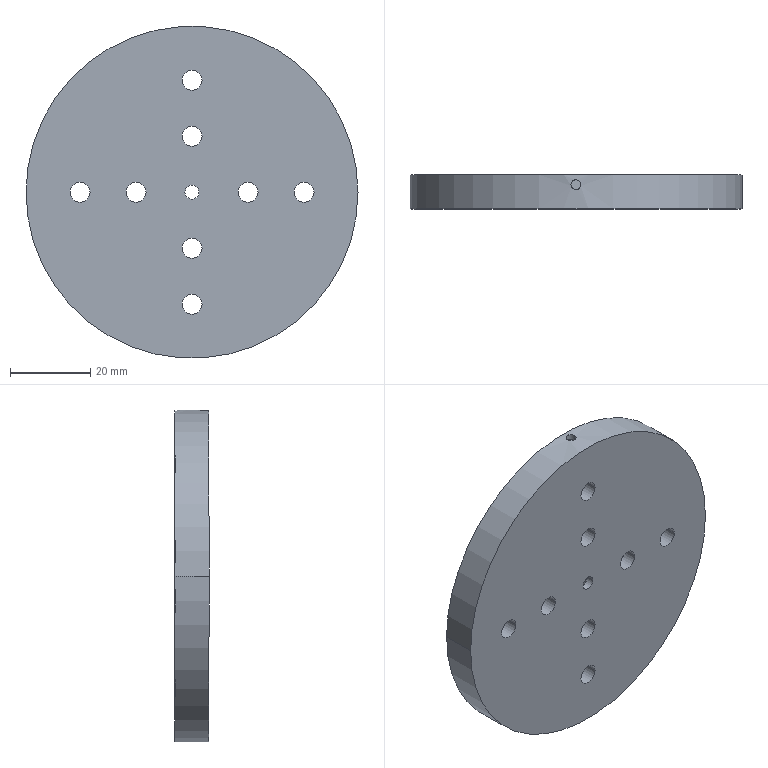Part | SolidWorks | features 3DProfileFeature 1, Chamfer 1, HoleWzd 1, ICE 1, Revolution 1 | 1 solid | 29 faces | box 83 x 8.5 x 83 mm | volume 20251 mm3 | cylinder 24 | plane 3 | cone 2 | commonest cylinder face diameters 5 x16 2.5 x2 3.5 x2 80 x2 83 x2
STEP:
#1=CARTESIAN_POINT('',(-1.25,6.,39.98));
#2=VERTEX_POINT('',#1);
#3=CARTESIAN_POINT('',(1.25,6.,39.98));
#4=VERTEX_POINT('',#3);
#5=CARTESIAN_POINT('',(-1.25,6.,39.98));
#6=CARTESIAN_POINT('',(-1.25,5.837,39.98));
#7=CARTESIAN_POINT('',(-1.217,5.672,39.982));
#8=CARTESIAN_POINT('',(-1.093,5.372,39.985));
#9=CARTESIAN_POINT('',(-0.9997,5.232,39.988));
#10=CARTESIAN_POINT('',(-0.7693,5.001,39.993));
#11=CARTESIAN_POINT('',(-0.6306,4.908,39.995));
#12=CARTESIAN_POINT('',(-0.3283,4.783,39.999));
#13=CARTESIAN_POINT('',(-0.1659,4.75,40.));
#14=CARTESIAN_POINT('',(0.1638,4.75,40.));
#15=CARTESIAN_POINT('',(0.3261,4.782,39.999));
#16=CARTESIAN_POINT('',(0.5535,4.876,39.996));
#17=CARTESIAN_POINT('',(0.6253,4.915,39.995));
#18=CARTESIAN_POINT('',(0.7611,5.005,39.993));
#19=CARTESIAN_POINT('',(0.8255,5.058,39.992));
#20=CARTESIAN_POINT('',(0.9987,5.231,39.988));
#21=CARTESIAN_POINT('',(1.092,5.37,39.985));
#22=CARTESIAN_POINT('',(1.217,5.671,39.982));
#23=CARTESIAN_POINT('',(1.25,5.835,39.98));
#24=CARTESIAN_POINT('',(1.25,6.,39.98));
#25=B_SPLINE_CURVE_WITH_KNOTS('',3,(#5,#6,#7,#8,#9,#10,#11,#12,#13,#14,#15,#16,#17,#18,#19,#20,#21,#22,#23,#24),.UNSPECIFIED.,.F.,.F.,(4,2,2,2,2,2,2,2,2,4),(0.003908,0.004397,0.004885,0.005374,0.005862,0.00635,0.006595,0.006839,0.007327,0.007816),.UNSPECIFIED.);
#26=EDGE_CURVE('',#2,#4,#25,.T.);
#27=ORIENTED_EDGE('',*,*,#26,.F.);
#28=CARTESIAN_POINT('',(-1.25,6.,41.481));
#29=VERTEX_POINT('',#28);
#30=CARTESIAN_POINT('',(-1.25,6.,41.5));
#31=DIRECTION('',(0.,0.,1.));
#32=VECTOR('',#31,1000.);
#33=LINE('',#30,#32);
#34=EDGE_CURVE('',#2,#29,#33,.T.);
#35=ORIENTED_EDGE('',*,*,#34,.T.);
#36=CARTESIAN_POINT('',(1.25,6.,41.481));
#37=VERTEX_POINT('',#36);
#38=CARTESIAN_POINT('',(1.25,6.,41.481));
#39=CARTESIAN_POINT('',(1.25,5.835,41.481));
#40=CARTESIAN_POINT('',(1.217,5.673,41.482));
#41=CARTESIAN_POINT('',(1.092,5.37,41.486));
#42=CARTESIAN_POINT('',(0.9991,5.231,41.488));
#43=CARTESIAN_POINT('',(0.7684,5.001,41.493));
#44=CARTESIAN_POINT('',(0.6289,4.908,41.496));
#45=CARTESIAN_POINT('',(0.328,4.783,41.499));
#46=CARTESIAN_POINT('',(0.1635,4.75,41.5));
#47=CARTESIAN_POINT('',(-0.1626,4.75,41.5));
#48=CARTESIAN_POINT('',(-0.3265,4.782,41.499));
#49=CARTESIAN_POINT('',(-0.6292,4.908,41.496));
#50=CARTESIAN_POINT('',(-0.767,4.999,41.493));
#51=CARTESIAN_POINT('',(-1.,5.233,41.488));
#52=CARTESIAN_POINT('',(-1.092,5.37,41.486));
#53=CARTESIAN_POINT('',(-1.186,5.597,41.483));
#54=CARTESIAN_POINT('',(-1.21,5.675,41.482));
#55=CARTESIAN_POINT('',(-1.242,5.836,41.481));
#56=CARTESIAN_POINT('',(-1.25,5.918,41.481));
#57=CARTESIAN_POINT('',(-1.25,6.,41.481));
#58=B_SPLINE_CURVE_WITH_KNOTS('',3,(#38,#39,#40,#41,#42,#43,#44,#45,#46,#47,#48,#49,#50,#51,#52,#53,#54,#55,#56,#57),.UNSPECIFIED.,.F.,.F.,(4,2,2,2,2,2,2,2,2,4),(0.,0.0004885,0.0009771,0.001466,0.001954,0.002443,0.002931,0.00342,0.003664,0.003908),.UNSPECIFIED.);
#59=EDGE_CURVE('',#37,#29,#58,.T.);
#60=ORIENTED_EDGE('',*,*,#59,.F.);
#61=CARTESIAN_POINT('',(1.25,6.,41.5));
#62=DIRECTION('',(0.,0.,1.));
#63=VECTOR('',#62,1000.);
#64=LINE('',#61,#63);
#65=EDGE_CURVE('',#4,#37,#64,.T.);
#66=ORIENTED_EDGE('',*,*,#65,.F.);
#67=EDGE_LOOP('',(#27,#35,#60,#66));
#68=FACE_OUTER_BOUND('',#67,.T.);
#69=CARTESIAN_POINT('',(0.,6.,41.5));
#70=DIRECTION('',(0.,0.,1.));
#71=DIRECTION('',(1.,0.,0.));
#72=AXIS2_PLACEMENT_3D('',#69,#70,#71);
#73=CYLINDRICAL_SURFACE('',#72,1.25);
#74=ADVANCED_FACE('',(#68),#73,.F.);
#75=CARTESIAN_POINT('',(-30.5,0.,0.));
#76=VERTEX_POINT('',#75);
#77=CARTESIAN_POINT('',(-25.5,0.,0.));
#78=VERTEX_POINT('',#77);
#79=CARTESIAN_POINT('',(-28.,0.,0.));
#80=DIRECTION('',(0.,-1.,0.));
#81=DIRECTION('',(-1.,0.,0.));
#82=AXIS2_PLACEMENT_3D('',#79,#80,#81);
#83=CIRCLE('',#82,2.5);
#84=EDGE_CURVE('',#76,#78,#83,.T.);
#85=ORIENTED_EDGE('',*,*,#84,.T.);
#86=CARTESIAN_POINT('',(-25.5,3.5,0.));
#87=VERTEX_POINT('',#86);
#88=CARTESIAN_POINT('',(-25.5,-0.001,0.));
#89=DIRECTION('',(0.,1.,0.));
#90=VECTOR('',#89,1000.);
#91=LINE('',#88,#90);
#92=EDGE_CURVE('',#78,#87,#91,.T.);
#93=ORIENTED_EDGE('',*,*,#92,.T.);
#94=CARTESIAN_POINT('',(-30.5,3.5,0.));
#95=VERTEX_POINT('',#94);
#96=CARTESIAN_POINT('',(-28.,3.5,0.));
#97=DIRECTION('',(0.,1.,0.));
#98=DIRECTION('',(-1.,0.,0.));
#99=AXIS2_PLACEMENT_3D('',#96,#97,#98);
#100=CIRCLE('',#99,2.5);
#101=EDGE_CURVE('',#87,#95,#100,.T.);
#102=ORIENTED_EDGE('',*,*,#101,.T.);
#103=CARTESIAN_POINT('',(-30.5,-0.001,0.));
#104=DIRECTION('',(0.,1.,0.));
#105=VECTOR('',#104,1000.);
#106=LINE('',#103,#105);
#107=EDGE_CURVE('',#76,#95,#106,.T.);
#108=ORIENTED_EDGE('',*,*,#107,.F.);
#109=EDGE_LOOP('',(#85,#93,#102,#108));
#110=FACE_OUTER_BOUND('',#109,.T.);
#111=CARTESIAN_POINT('',(-28.,-0.001,0.));
#112=DIRECTION('',(0.,1.,0.));
#113=DIRECTION('',(-1.,0.,0.));
#114=AXIS2_PLACEMENT_3D('',#111,#112,#113);
#115=CYLINDRICAL_SURFACE('',#114,2.5);
#116=ADVANCED_FACE('',(#110),#115,.F.);
#117=CARTESIAN_POINT('',(-16.5,0.,0.));
#118=VERTEX_POINT('',#117);
#119=CARTESIAN_POINT('',(-11.5,0.,0.));
#120=VERTEX_POINT('',#119);
#121=CARTESIAN_POINT('',(-14.,0.,0.));
#122=DIRECTION('',(0.,-1.,0.));
#123=DIRECTION('',(-1.,0.,0.));
#124=AXIS2_PLACEMENT_3D('',#121,#122,#123);
#125=CIRCLE('',#124,2.5);
#126=EDGE_CURVE('',#118,#120,#125,.T.);
#127=ORIENTED_EDGE('',*,*,#126,.T.);
#128=CARTESIAN_POINT('',(-11.5,3.5,0.));
#129=VERTEX_POINT('',#128);
#130=CARTESIAN_POINT('',(-11.5,-0.001,0.));
#131=DIRECTION('',(0.,1.,0.));
#132=VECTOR('',#131,1000.);
#133=LINE('',#130,#132);
#134=EDGE_CURVE('',#120,#129,#133,.T.);
#135=ORIENTED_EDGE('',*,*,#134,.T.);
#136=CARTESIAN_POINT('',(-16.5,3.5,0.));
#137=VERTEX_POINT('',#136);
#138=CARTESIAN_POINT('',(-14.,3.5,0.));
#139=DIRECTION('',(0.,1.,0.));
#140=DIRECTION('',(-1.,0.,0.));
#141=AXIS2_PLACEMENT_3D('',#138,#139,#140);
#142=CIRCLE('',#141,2.5);
#143=EDGE_CURVE('',#129,#137,#142,.T.);
#144=ORIENTED_EDGE('',*,*,#143,.T.);
#145=CARTESIAN_POINT('',(-16.5,-0.001,0.));
#146=DIRECTION('',(0.,1.,0.));
#147=VECTOR('',#146,1000.);
#148=LINE('',#145,#147);
#149=EDGE_CURVE('',#118,#137,#148,.T.);
#150=ORIENTED_EDGE('',*,*,#149,.F.);
#151=EDGE_LOOP('',(#127,#135,#144,#150));
#152=FACE_OUTER_BOUND('',#151,.T.);
#153=CARTESIAN_POINT('',(-14.,-0.001,0.));
#154=DIRECTION('',(0.,1.,0.));
#155=DIRECTION('',(-1.,0.,0.));
#156=AXIS2_PLACEMENT_3D('',#153,#154,#155);
#157=CYLINDRICAL_SURFACE('',#156,2.5);
#158=ADVANCED_FACE('',(#152),#157,.F.);
#159=CARTESIAN_POINT('',(-2.5,0.,28.));
#160=VERTEX_POINT('',#159);
#161=CARTESIAN_POINT('',(2.5,0.,28.));
#162=VERTEX_POINT('',#161);
#163=CARTESIAN_POINT('',(0.,0.,28.));
#164=DIRECTION('',(0.,-1.,0.));
#165=DIRECTION('',(-1.,0.,0.));
#166=AXIS2_PLACEMENT_3D('',#163,#164,#165);
#167=CIRCLE('',#166,2.5);
#168=EDGE_CURVE('',#160,#162,#167,.T.);
#169=ORIENTED_EDGE('',*,*,#168,.T.);
#170=CARTESIAN_POINT('',(2.5,3.5,28.));
#171=VERTEX_POINT('',#170);
#172=CARTESIAN_POINT('',(2.5,-0.001,28.));
#173=DIRECTION('',(0.,1.,0.));
#174=VECTOR('',#173,1000.);
#175=LINE('',#172,#174);
#176=EDGE_CURVE('',#162,#171,#175,.T.);
#177=ORIENTED_EDGE('',*,*,#176,.T.);
#178=CARTESIAN_POINT('',(-2.5,3.5,28.));
#179=VERTEX_POINT('',#178);
#180=CARTESIAN_POINT('',(0.,3.5,28.));
#181=DIRECTION('',(0.,1.,0.));
#182=DIRECTION('',(-1.,0.,0.));
#183=AXIS2_PLACEMENT_3D('',#180,#181,#182);
#184=CIRCLE('',#183,2.5);
#185=EDGE_CURVE('',#171,#179,#184,.T.);
#186=ORIENTED_EDGE('',*,*,#185,.T.);
#187=CARTESIAN_POINT('',(-2.5,-0.001,28.));
#188=DIRECTION('',(0.,1.,0.));
#189=VECTOR('',#188,1000.);
#190=LINE('',#187,#189);
#191=EDGE_CURVE('',#160,#179,#190,.T.);
#192=ORIENTED_EDGE('',*,*,#191,.F.);
#193=EDGE_LOOP('',(#169,#177,#186,#192));
#194=FACE_OUTER_BOUND('',#193,.T.);
#195=CARTESIAN_POINT('',(0.,-0.001,28.));
#196=DIRECTION('',(0.,1.,0.));
#197=DIRECTION('',(-1.,0.,0.));
#198=AXIS2_PLACEMENT_3D('',#195,#196,#197);
#199=CYLINDRICAL_SURFACE('',#198,2.5);
#200=ADVANCED_FACE('',(#194),#199,.F.);
#201=CARTESIAN_POINT('',(-2.5,0.,14.));
#202=VERTEX_POINT('',#201);
#203=CARTESIAN_POINT('',(2.5,0.,14.));
#204=VERTEX_POINT('',#203);
#205=CARTESIAN_POINT('',(0.,0.,14.));
#206=DIRECTION('',(0.,-1.,0.));
#207=DIRECTION('',(-1.,0.,0.));
#208=AXIS2_PLACEMENT_3D('',#205,#206,#207);
#209=CIRCLE('',#208,2.5);
#210=EDGE_CURVE('',#202,#204,#209,.T.);
#211=ORIENTED_EDGE('',*,*,#210,.T.);
#212=CARTESIAN_POINT('',(2.5,3.5,14.));
#213=VERTEX_POINT('',#212);
#214=CARTESIAN_POINT('',(2.5,-0.001,14.));
#215=DIRECTION('',(0.,1.,0.));
#216=VECTOR('',#215,1000.);
#217=LINE('',#214,#216);
#218=EDGE_CURVE('',#204,#213,#217,.T.);
#219=ORIENTED_EDGE('',*,*,#218,.T.);
#220=CARTESIAN_POINT('',(-2.5,3.5,14.));
#221=VERTEX_POINT('',#220);
#222=CARTESIAN_POINT('',(0.,3.5,14.));
#223=DIRECTION('',(0.,1.,0.));
#224=DIRECTION('',(-1.,0.,0.));
#225=AXIS2_PLACEMENT_3D('',#222,#223,#224);
#226=CIRCLE('',#225,2.5);
#227=EDGE_CURVE('',#213,#221,#226,.T.);
#228=ORIENTED_EDGE('',*,*,#227,.T.);
#229=CARTESIAN_POINT('',(-2.5,-0.001,14.));
#230=DIRECTION('',(0.,1.,0.));
#231=VECTOR('',#230,1000.);
#232=LINE('',#229,#231);
#233=EDGE_CURVE('',#202,#221,#232,.T.);
#234=ORIENTED_EDGE('',*,*,#233,.F.);
#235=EDGE_LOOP('',(#211,#219,#228,#234));
#236=FACE_OUTER_BOUND('',#235,.T.);
#237=CARTESIAN_POINT('',(0.,-0.001,14.));
#238=DIRECTION('',(0.,1.,0.));
#239=DIRECTION('',(-1.,0.,0.));
#240=AXIS2_PLACEMENT_3D('',#237,#238,#239);
#241=CYLINDRICAL_SURFACE('',#240,2.5);
#242=ADVANCED_FACE('',(#236),#241,.F.);
#243=CARTESIAN_POINT('',(25.5,0.,0.));
#244=VERTEX_POINT('',#243);
#245=CARTESIAN_POINT('',(30.5,0.,0.));
#246=VERTEX_POINT('',#245);
#247=CARTESIAN_POINT('',(28.,0.,0.));
#248=DIRECTION('',(0.,-1.,0.));
#249=DIRECTION('',(-1.,0.,0.));
#250=AXIS2_PLACEMENT_3D('',#247,#248,#249);
#251=CIRCLE('',#250,2.5);
#252=EDGE_CURVE('',#244,#246,#251,.T.);
#253=ORIENTED_EDGE('',*,*,#252,.T.);
#254=CARTESIAN_POINT('',(30.5,3.5,0.));
#255=VERTEX_POINT('',#254);
#256=CARTESIAN_POINT('',(30.5,-0.001,0.));
#257=DIRECTION('',(0.,1.,0.));
#258=VECTOR('',#257,1000.);
#259=LINE('',#256,#258);
#260=EDGE_CURVE('',#246,#255,#259,.T.);
#261=ORIENTED_EDGE('',*,*,#260,.T.);
#262=CARTESIAN_POINT('',(25.5,3.5,0.));
#263=VERTEX_POINT('',#262);
#264=CARTESIAN_POINT('',(28.,3.5,0.));
#265=DIRECTION('',(0.,1.,0.));
#266=DIRECTION('',(-1.,0.,0.));
#267=AXIS2_PLACEMENT_3D('',#264,#265,#266);
#268=CIRCLE('',#267,2.5);
#269=EDGE_CURVE('',#255,#263,#268,.T.);
#270=ORIENTED_EDGE('',*,*,#269,.T.);
#271=CARTESIAN_POINT('',(25.5,-0.001,0.));
#272=DIRECTION('',(0.,1.,0.));
#273=VECTOR('',#272,1000.);
#274=LINE('',#271,#273);
#275=EDGE_CURVE('',#244,#263,#274,.T.);
#276=ORIENTED_EDGE('',*,*,#275,.F.);
#277=EDGE_LOOP('',(#253,#261,#270,#276));
#278=FACE_OUTER_BOUND('',#277,.T.);
#279=CARTESIAN_POINT('',(28.,-0.001,0.));
#280=DIRECTION('',(0.,1.,0.));
#281=DIRECTION('',(-1.,0.,0.));
#282=AXIS2_PLACEMENT_3D('',#279,#280,#281);
#283=CYLINDRICAL_SURFACE('',#282,2.5);
#284=ADVANCED_FACE('',(#278),#283,.F.);
#285=CARTESIAN_POINT('',(11.5,0.,0.));
#286=VERTEX_POINT('',#285);
#287=CARTESIAN_POINT('',(16.5,0.,0.));
#288=VERTEX_POINT('',#287);
#289=CARTESIAN_POINT('',(14.,0.,0.));
#290=DIRECTION('',(0.,-1.,0.));
#291=DIRECTION('',(-1.,0.,0.));
#292=AXIS2_PLACEMENT_3D('',#289,#290,#291);
#293=CIRCLE('',#292,2.5);
#294=EDGE_CURVE('',#286,#288,#293,.T.);
#295=ORIENTED_EDGE('',*,*,#294,.T.);
#296=CARTESIAN_POINT('',(16.5,3.5,0.));
#297=VERTEX_POINT('',#296);
#298=CARTESIAN_POINT('',(16.5,-0.001,0.));
#299=DIRECTION('',(0.,1.,0.));
#300=VECTOR('',#299,1000.);
#301=LINE('',#298,#300);
#302=EDGE_CURVE('',#288,#297,#301,.T.);
#303=ORIENTED_EDGE('',*,*,#302,.T.);
#304=CARTESIAN_POINT('',(11.5,3.5,0.));
#305=VERTEX_POINT('',#304);
#306=CARTESIAN_POINT('',(14.,3.5,0.));
#307=DIRECTION('',(0.,1.,0.));
#308=DIRECTION('',(-1.,0.,0.));
#309=AXIS2_PLACEMENT_3D('',#306,#307,#308);
#310=CIRCLE('',#309,2.5);
#311=EDGE_CURVE('',#297,#305,#310,.T.);
#312=ORIENTED_EDGE('',*,*,#311,.T.);
#313=CARTESIAN_POINT('',(11.5,-0.001,0.));
#314=DIRECTION('',(0.,1.,0.));
#315=VECTOR('',#314,1000.);
#316=LINE('',#313,#315);
#317=EDGE_CURVE('',#286,#305,#316,.T.);
#318=ORIENTED_EDGE('',*,*,#317,.F.);
#319=EDGE_LOOP('',(#295,#303,#312,#318));
#320=FACE_OUTER_BOUND('',#319,.T.);
#321=CARTESIAN_POINT('',(14.,-0.001,0.));
#322=DIRECTION('',(0.,1.,0.));
#323=DIRECTION('',(-1.,0.,0.));
#324=AXIS2_PLACEMENT_3D('',#321,#322,#323);
#325=CYLINDRICAL_SURFACE('',#324,2.5);
#326=ADVANCED_FACE('',(#320),#325,.F.);
#327=CARTESIAN_POINT('',(-2.5,0.,-28.));
#328=VERTEX_POINT('',#327);
#329=CARTESIAN_POINT('',(2.5,0.,-28.));
#330=VERTEX_POINT('',#329);
#331=CARTESIAN_POINT('',(0.,0.,-28.));
#332=DIRECTION('',(0.,-1.,0.));
#333=DIRECTION('',(-1.,0.,0.));
#334=AXIS2_PLACEMENT_3D('',#331,#332,#333);
#335=CIRCLE('',#334,2.5);
#336=EDGE_CURVE('',#328,#330,#335,.T.);
#337=ORIENTED_EDGE('',*,*,#336,.T.);
#338=CARTESIAN_POINT('',(2.5,3.5,-28.));
#339=VERTEX_POINT('',#338);
#340=CARTESIAN_POINT('',(2.5,-0.001,-28.));
#341=DIRECTION('',(0.,1.,0.));
#342=VECTOR('',#341,1000.);
#343=LINE('',#340,#342);
#344=EDGE_CURVE('',#330,#339,#343,.T.);
#345=ORIENTED_EDGE('',*,*,#344,.T.);
#346=CARTESIAN_POINT('',(-2.5,3.5,-28.));
#347=VERTEX_POINT('',#346);
#348=CARTESIAN_POINT('',(0.,3.5,-28.));
#349=DIRECTION('',(0.,1.,0.));
#350=DIRECTION('',(-1.,0.,0.));
#351=AXIS2_PLACEMENT_3D('',#348,#349,#350);
#352=CIRCLE('',#351,2.5);
#353=EDGE_CURVE('',#339,#347,#352,.T.);
#354=ORIENTED_EDGE('',*,*,#353,.T.);
#355=CARTESIAN_POINT('',(-2.5,-0.001,-28.));
#356=DIRECTION('',(0.,1.,0.));
#357=VECTOR('',#356,1000.);
#358=LINE('',#355,#357);
#359=EDGE_CURVE('',#328,#347,#358,.T.);
#360=ORIENTED_EDGE('',*,*,#359,.F.);
#361=EDGE_LOOP('',(#337,#345,#354,#360));
#362=FACE_OUTER_BOUND('',#361,.T.);
#363=CARTESIAN_POINT('',(0.,-0.001,-28.));
#364=DIRECTION('',(0.,1.,0.));
#365=DIRECTION('',(-1.,0.,0.));
#366=AXIS2_PLACEMENT_3D('',#363,#364,#365);
#367=CYLINDRICAL_SURFACE('',#366,2.5);
#368=ADVANCED_FACE('',(#362),#367,.F.);
#369=CARTESIAN_POINT('',(-2.5,0.,-14.));
#370=VERTEX_POINT('',#369);
#371=CARTESIAN_POINT('',(2.5,0.,-14.));
#372=VERTEX_POINT('',#371);
#373=CARTESIAN_POINT('',(0.,0.,-14.));
#374=DIRECTION('',(0.,-1.,0.));
#375=DIRECTION('',(-1.,0.,0.));
#376=AXIS2_PLACEMENT_3D('',#373,#374,#375);
#377=CIRCLE('',#376,2.5);
#378=EDGE_CURVE('',#370,#372,#377,.T.);
#379=ORIENTED_EDGE('',*,*,#378,.T.);
#380=CARTESIAN_POINT('',(2.5,3.5,-14.));
#381=VERTEX_POINT('',#380);
#382=CARTESIAN_POINT('',(2.5,-0.001,-14.));
#383=DIRECTION('',(0.,1.,0.));
#384=VECTOR('',#383,1000.);
#385=LINE('',#382,#384);
#386=EDGE_CURVE('',#372,#381,#385,.T.);
#387=ORIENTED_EDGE('',*,*,#386,.T.);
#388=CARTESIAN_POINT('',(-2.5,3.5,-14.));
#389=VERTEX_POINT('',#388);
#390=CARTESIAN_POINT('',(0.,3.5,-14.));
#391=DIRECTION('',(0.,1.,0.));
#392=DIRECTION('',(-1.,0.,0.));
#393=AXIS2_PLACEMENT_3D('',#390,#391,#392);
#394=CIRCLE('',#393,2.5);
#395=EDGE_CURVE('',#381,#389,#394,.T.);
#396=ORIENTED_EDGE('',*,*,#395,.T.);
#397=CARTESIAN_POINT('',(-2.5,-0.001,-14.));
#398=DIRECTION('',(0.,1.,0.));
#399=VECTOR('',#398,1000.);
#400=LINE('',#397,#399);
#401=EDGE_CURVE('',#370,#389,#400,.T.);
#402=ORIENTED_EDGE('',*,*,#401,.F.);
#403=EDGE_LOOP('',(#379,#387,#396,#402));
#404=FACE_OUTER_BOUND('',#403,.T.);
#405=CARTESIAN_POINT('',(0.,-0.001,-14.));
#406=DIRECTION('',(0.,1.,0.));
#407=DIRECTION('',(-1.,0.,0.));
#408=AXIS2_PLACEMENT_3D('',#405,#406,#407);
#409=CYLINDRICAL_SURFACE('',#408,2.5);
#410=ADVANCED_FACE('',(#404),#409,.F.);
#411=ORIENTED_EDGE('',*,*,#59,.T.);
#412=CARTESIAN_POINT('',(-1.25,6.,41.481));
#413=CARTESIAN_POINT('',(-1.25,6.163,41.481));
#414=CARTESIAN_POINT('',(-1.217,6.328,41.482));
#415=CARTESIAN_POINT('',(-1.093,6.628,41.486));
#416=CARTESIAN_POINT('',(-0.9997,6.768,41.488));
#417=CARTESIAN_POINT('',(-0.7693,6.999,41.493));
#418=CARTESIAN_POINT('',(-0.6306,7.092,41.495));
#419=CARTESIAN_POINT('',(-0.3283,7.217,41.499));
#420=CARTESIAN_POINT('',(-0.1659,7.25,41.5));
#421=CARTESIAN_POINT('',(0.1638,7.25,41.5));
#422=CARTESIAN_POINT('',(0.3261,7.218,41.499));
#423=CARTESIAN_POINT('',(0.5535,7.124,41.496));
#424=CARTESIAN_POINT('',(0.6253,7.085,41.495));
#425=CARTESIAN_POINT('',(0.7611,6.995,41.493));
#426=CARTESIAN_POINT('',(0.8255,6.942,41.492));
#427=CARTESIAN_POINT('',(0.9987,6.769,41.488));
#428=CARTESIAN_POINT('',(1.092,6.63,41.486));
#429=CARTESIAN_POINT('',(1.217,6.329,41.482));
#430=CARTESIAN_POINT('',(1.25,6.165,41.481));
#431=CARTESIAN_POINT('',(1.25,6.,41.481));
#432=B_SPLINE_CURVE_WITH_KNOTS('',3,(#412,#413,#414,#415,#416,#417,#418,#419,#420,#421,#422,#423,#424,#425,#426,#427,#428,#429,#430,#431),.UNSPECIFIED.,.F.,.F.,(4,2,2,2,2,2,2,2,2,4),(0.003908,0.004397,0.004885,0.005374,0.005862,0.00635,0.006595,0.006839,0.007327,0.007816),.UNSPECIFIED.);
#433=EDGE_CURVE('',#29,#37,#432,.T.);
#434=ORIENTED_EDGE('',*,*,#433,.T.);
#435=EDGE_LOOP('',(#411,#434));
#436=FACE_BOUND('',#435,.T.);
#437=CARTESIAN_POINT('',(-41.5,0.,0.));
#438=VERTEX_POINT('',#437);
#439=CARTESIAN_POINT('',(41.5,0.,0.));
#440=VERTEX_POINT('',#439);
#441=CARTESIAN_POINT('',(0.,0.,0.));
#442=DIRECTION('',(0.,1.,0.));
#443=DIRECTION('',(-1.,0.,0.));
#444=AXIS2_PLACEMENT_3D('',#441,#442,#443);
#445=CIRCLE('',#444,41.5);
#446=EDGE_CURVE('',#438,#440,#445,.T.);
#447=ORIENTED_EDGE('',*,*,#446,.T.);
#448=CARTESIAN_POINT('',(41.5,8.5,0.));
#449=VERTEX_POINT('',#448);
#450=CARTESIAN_POINT('',(41.5,9.31,0.));
#451=DIRECTION('',(0.,1.,0.));
#452=VECTOR('',#451,1000.);
#453=LINE('',#450,#452);
#454=EDGE_CURVE('',#440,#449,#453,.T.);
#455=ORIENTED_EDGE('',*,*,#454,.T.);
#456=CARTESIAN_POINT('',(-41.5,8.5,0.));
#457=VERTEX_POINT('',#456);
#458=CARTESIAN_POINT('',(0.,8.5,0.));
#459=DIRECTION('',(0.,1.,0.));
#460=DIRECTION('',(-1.,0.,0.));
#461=AXIS2_PLACEMENT_3D('',#458,#459,#460);
#462=CIRCLE('',#461,41.5);
#463=EDGE_CURVE('',#457,#449,#462,.T.);
#464=ORIENTED_EDGE('',*,*,#463,.F.);
#465=CARTESIAN_POINT('',(-41.5,9.31,0.));
#466=DIRECTION('',(0.,1.,0.));
#467=VECTOR('',#466,1000.);
#468=LINE('',#465,#467);
#469=EDGE_CURVE('',#438,#457,#468,.T.);
#470=ORIENTED_EDGE('',*,*,#469,.F.);
#471=EDGE_LOOP('',(#447,#455,#464,#470));
#472=FACE_OUTER_BOUND('',#471,.T.);
#473=CARTESIAN_POINT('',(0.,9.31,0.));
#474=DIRECTION('',(0.,1.,0.));
#475=DIRECTION('',(-1.,0.,0.));
#476=AXIS2_PLACEMENT_3D('',#473,#474,#475);
#477=CYLINDRICAL_SURFACE('',#476,41.5);
#478=ADVANCED_FACE('',(#436,#472),#477,.T.);
#479=CARTESIAN_POINT('',(40.,3.5,0.));
#480=VERTEX_POINT('',#479);
#481=CARTESIAN_POINT('',(-40.,3.5,0.));
#482=VERTEX_POINT('',#481);
#483=CARTESIAN_POINT('',(0.,3.5,0.));
#484=DIRECTION('',(0.,1.,0.));
#485=DIRECTION('',(-1.,0.,0.));
#486=AXIS2_PLACEMENT_3D('',#483,#484,#485);
#487=CIRCLE('',#486,40.);
#488=EDGE_CURVE('',#480,#482,#487,.T.);
#489=ORIENTED_EDGE('',*,*,#488,.F.);
#490=CARTESIAN_POINT('',(40.,8.5,0.));
#491=VERTEX_POINT('',#490);
#492=CARTESIAN_POINT('',(40.,9.31,0.));
#493=DIRECTION('',(0.,1.,0.));
#494=VECTOR('',#493,1000.);
#495=LINE('',#492,#494);
#496=EDGE_CURVE('',#480,#491,#495,.T.);
#497=ORIENTED_EDGE('',*,*,#496,.T.);
#498=CARTESIAN_POINT('',(-40.,8.5,0.));
#499=VERTEX_POINT('',#498);
#500=CARTESIAN_POINT('',(0.,8.5,0.));
#501=DIRECTION('',(0.,1.,0.));
#502=DIRECTION('',(-1.,0.,0.));
#503=AXIS2_PLACEMENT_3D('',#500,#501,#502);
#504=CIRCLE('',#503,40.);
#505=EDGE_CURVE('',#491,#499,#504,.T.);
#506=ORIENTED_EDGE('',*,*,#505,.T.);
#507=CARTESIAN_POINT('',(-40.,9.31,0.));
#508=DIRECTION('',(0.,1.,0.));
#509=VECTOR('',#508,1000.);
#510=LINE('',#507,#509);
#511=EDGE_CURVE('',#482,#499,#510,.T.);
#512=ORIENTED_EDGE('',*,*,#511,.F.);
#513=EDGE_LOOP('',(#489,#497,#506,#512));
#514=FACE_OUTER_BOUND('',#513,.T.);
#515=CARTESIAN_POINT('',(0.,9.31,0.));
#516=DIRECTION('',(0.,1.,0.));
#517=DIRECTION('',(-1.,0.,0.));
#518=AXIS2_PLACEMENT_3D('',#515,#516,#517);
#519=CYLINDRICAL_SURFACE('',#518,40.);
#520=ADVANCED_FACE('',(#514),#519,.F.);
#521=CARTESIAN_POINT('',(1.75,2.,0.));
#522=VERTEX_POINT('',#521);
#523=CARTESIAN_POINT('',(-1.75,2.,0.));
#524=VERTEX_POINT('',#523);
#525=CARTESIAN_POINT('',(0.,2.,0.));
#526=DIRECTION('',(0.,1.,0.));
#527=DIRECTION('',(-1.,0.,0.));
#528=AXIS2_PLACEMENT_3D('',#525,#526,#527);
#529=CIRCLE('',#528,1.75);
#530=EDGE_CURVE('',#522,#524,#529,.T.);
#531=ORIENTED_EDGE('',*,*,#530,.F.);
#532=CARTESIAN_POINT('',(3.25,3.5,0.));
#533=VERTEX_POINT('',#532);
#534=CARTESIAN_POINT('',(3.25,3.5,0.));
#535=DIRECTION('',(0.7071,0.7071,0.));
#536=VECTOR('',#535,1000.);
#537=LINE('',#534,#536);
#538=EDGE_CURVE('',#522,#533,#537,.T.);
#539=ORIENTED_EDGE('',*,*,#538,.T.);
#540=CARTESIAN_POINT('',(-3.25,3.5,0.));
#541=VERTEX_POINT('',#540);
#542=CARTESIAN_POINT('',(0.,3.5,0.));
#543=DIRECTION('',(0.,1.,0.));
#544=DIRECTION('',(-1.,0.,0.));
#545=AXIS2_PLACEMENT_3D('',#542,#543,#544);
#546=CIRCLE('',#545,3.25);
#547=EDGE_CURVE('',#533,#541,#546,.T.);
#548=ORIENTED_EDGE('',*,*,#547,.T.);
#549=CARTESIAN_POINT('',(-3.25,3.5,0.));
#550=DIRECTION('',(-0.7071,0.7071,0.));
#551=VECTOR('',#550,1000.);
#552=LINE('',#549,#551);
#553=EDGE_CURVE('',#524,#541,#552,.T.);
#554=ORIENTED_EDGE('',*,*,#553,.F.);
#555=EDGE_LOOP('',(#531,#539,#548,#554));
#556=FACE_OUTER_BOUND('',#555,.T.);
#557=CARTESIAN_POINT('',(0.,3.5,0.));
#558=DIRECTION('',(0.,1.,0.));
#559=DIRECTION('',(-1.,0.,0.));
#560=AXIS2_PLACEMENT_3D('',#557,#558,#559);
#561=CONICAL_SURFACE('',#560,3.25,0.7854);
#562=ADVANCED_FACE('',(#556),#561,.F.);
#563=CARTESIAN_POINT('',(1.75,0.,0.));
#564=VERTEX_POINT('',#563);
#565=CARTESIAN_POINT('',(-1.75,0.,0.));
#566=VERTEX_POINT('',#565);
#567=CARTESIAN_POINT('',(0.,0.,0.));
#568=DIRECTION('',(0.,1.,0.));
#569=DIRECTION('',(-1.,0.,0.));
#570=AXIS2_PLACEMENT_3D('',#567,#568,#569);
#571=CIRCLE('',#570,1.75);
#572=EDGE_CURVE('',#564,#566,#571,.T.);
#573=ORIENTED_EDGE('',*,*,#572,.F.);
#574=CARTESIAN_POINT('',(1.75,9.31,0.));
#575=DIRECTION('',(0.,1.,0.));
#576=VECTOR('',#575,1000.);
#577=LINE('',#574,#576);
#578=EDGE_CURVE('',#564,#522,#577,.T.);
#579=ORIENTED_EDGE('',*,*,#578,.T.);
#580=ORIENTED_EDGE('',*,*,#530,.T.);
#581=CARTESIAN_POINT('',(-1.75,9.31,0.));
#582=DIRECTION('',(0.,1.,0.));
#583=VECTOR('',#582,1000.);
#584=LINE('',#581,#583);
#585=EDGE_CURVE('',#566,#524,#584,.T.);
#586=ORIENTED_EDGE('',*,*,#585,.F.);
#587=EDGE_LOOP('',(#573,#579,#580,#586));
#588=FACE_OUTER_BOUND('',#587,.T.);
#589=CARTESIAN_POINT('',(0.,9.31,0.));
#590=DIRECTION('',(0.,1.,0.));
#591=DIRECTION('',(-1.,0.,0.));
#592=AXIS2_PLACEMENT_3D('',#589,#590,#591);
#593=CYLINDRICAL_SURFACE('',#592,1.75);
#594=ADVANCED_FACE('',(#588),#593,.F.);
#595=ORIENTED_EDGE('',*,*,#84,.F.);
#596=CARTESIAN_POINT('',(-28.,0.,0.));
#597=DIRECTION('',(0.,-1.,0.));
#598=DIRECTION('',(-1.,0.,0.));
#599=AXIS2_PLACEMENT_3D('',#596,#597,#598);
#600=CIRCLE('',#599,2.5);
#601=EDGE_CURVE('',#78,#76,#600,.T.);
#602=ORIENTED_EDGE('',*,*,#601,.F.);
#603=EDGE_LOOP('',(#595,#602));
#604=FACE_BOUND('',#603,.T.);
#605=ORIENTED_EDGE('',*,*,#126,.F.);
#606=CARTESIAN_POINT('',(-14.,0.,0.));
#607=DIRECTION('',(0.,-1.,0.));
#608=DIRECTION('',(-1.,0.,0.));
#609=AXIS2_PLACEMENT_3D('',#606,#607,#608);
#610=CIRCLE('',#609,2.5);
#611=EDGE_CURVE('',#120,#118,#610,.T.);
#612=ORIENTED_EDGE('',*,*,#611,.F.);
#613=EDGE_LOOP('',(#605,#612));
#614=FACE_BOUND('',#613,.T.);
#615=ORIENTED_EDGE('',*,*,#168,.F.);
#616=CARTESIAN_POINT('',(0.,0.,28.));
#617=DIRECTION('',(0.,-1.,0.));
#618=DIRECTION('',(-1.,0.,0.));
#619=AXIS2_PLACEMENT_3D('',#616,#617,#618);
#620=CIRCLE('',#619,2.5);
#621=EDGE_CURVE('',#162,#160,#620,.T.);
#622=ORIENTED_EDGE('',*,*,#621,.F.);
#623=EDGE_LOOP('',(#615,#622));
#624=FACE_BOUND('',#623,.T.);
#625=ORIENTED_EDGE('',*,*,#210,.F.);
#626=CARTESIAN_POINT('',(0.,0.,14.));
#627=DIRECTION('',(0.,-1.,0.));
#628=DIRECTION('',(-1.,0.,0.));
#629=AXIS2_PLACEMENT_3D('',#626,#627,#628);
#630=CIRCLE('',#629,2.5);
#631=EDGE_CURVE('',#204,#202,#630,.T.);
#632=ORIENTED_EDGE('',*,*,#631,.F.);
#633=EDGE_LOOP('',(#625,#632));
#634=FACE_BOUND('',#633,.T.);
#635=ORIENTED_EDGE('',*,*,#252,.F.);
#636=CARTESIAN_POINT('',(28.,0.,0.));
#637=DIRECTION('',(0.,-1.,0.));
#638=DIRECTION('',(-1.,0.,0.));
#639=AXIS2_PLACEMENT_3D('',#636,#637,#638);
#640=CIRCLE('',#639,2.5);
#641=EDGE_CURVE('',#246,#244,#640,.T.);
#642=ORIENTED_EDGE('',*,*,#641,.F.);
#643=EDGE_LOOP('',(#635,#642));
#644=FACE_BOUND('',#643,.T.);
#645=ORIENTED_EDGE('',*,*,#294,.F.);
#646=CARTESIAN_POINT('',(14.,0.,0.));
#647=DIRECTION('',(0.,-1.,0.));
#648=DIRECTION('',(-1.,0.,0.));
#649=AXIS2_PLACEMENT_3D('',#646,#647,#648);
#650=CIRCLE('',#649,2.5);
#651=EDGE_CURVE('',#288,#286,#650,.T.);
#652=ORIENTED_EDGE('',*,*,#651,.F.);
#653=EDGE_LOOP('',(#645,#652));
#654=FACE_BOUND('',#653,.T.);
#655=ORIENTED_EDGE('',*,*,#336,.F.);
#656=CARTESIAN_POINT('',(0.,0.,-28.));
#657=DIRECTION('',(0.,-1.,0.));
#658=DIRECTION('',(-1.,0.,0.));
#659=AXIS2_PLACEMENT_3D('',#656,#657,#658);
#660=CIRCLE('',#659,2.5);
#661=EDGE_CURVE('',#330,#328,#660,.T.);
#662=ORIENTED_EDGE('',*,*,#661,.F.);
#663=EDGE_LOOP('',(#655,#662));
#664=FACE_BOUND('',#663,.T.);
#665=ORIENTED_EDGE('',*,*,#378,.F.);
#666=CARTESIAN_POINT('',(0.,0.,-14.));
#667=DIRECTION('',(0.,-1.,0.));
#668=DIRECTION('',(-1.,0.,0.));
#669=AXIS2_PLACEMENT_3D('',#666,#667,#668);
#670=CIRCLE('',#669,2.5);
#671=EDGE_CURVE('',#372,#370,#670,.T.);
#672=ORIENTED_EDGE('',*,*,#671,.F.);
#673=EDGE_LOOP('',(#665,#672));
#674=FACE_BOUND('',#673,.T.);
#675=ORIENTED_EDGE('',*,*,#446,.F.);
#676=CARTESIAN_POINT('',(0.,0.,0.));
#677=DIRECTION('',(0.,1.,0.));
#678=DIRECTION('',(-1.,0.,0.));
#679=AXIS2_PLACEMENT_3D('',#676,#677,#678);
#680=CIRCLE('',#679,41.5);
#681=EDGE_CURVE('',#440,#438,#680,.T.);
#682=ORIENTED_EDGE('',*,*,#681,.F.);
#683=EDGE_LOOP('',(#675,#682));
#684=FACE_OUTER_BOUND('',#683,.T.);
#685=CARTESIAN_POINT('',(0.,0.,0.));
#686=DIRECTION('',(0.,1.,0.));
#687=DIRECTION('',(-1.,0.,0.));
#688=AXIS2_PLACEMENT_3D('',#685,#686,#687);
#689=CIRCLE('',#688,1.75);
#690=EDGE_CURVE('',#566,#564,#689,.T.);
#691=ORIENTED_EDGE('',*,*,#690,.T.);
#692=ORIENTED_EDGE('',*,*,#572,.T.);
#693=EDGE_LOOP('',(#691,#692));
#694=FACE_BOUND('',#693,.T.);
#695=CARTESIAN_POINT('',(41.5,0.,0.));
#696=DIRECTION('',(0.,1.,0.));
#697=DIRECTION('',(-1.,0.,0.));
#698=AXIS2_PLACEMENT_3D('',#695,#696,#697);
#699=PLANE('',#698);
#700=ADVANCED_FACE('',(#604,#614,#624,#634,#644,#654,#664,#674,#684,#694),#699,.F.);
#701=ORIENTED_EDGE('',*,*,#578,.F.);
#702=ORIENTED_EDGE('',*,*,#690,.F.);
#703=ORIENTED_EDGE('',*,*,#585,.T.);
#704=CARTESIAN_POINT('',(0.,2.,0.));
#705=DIRECTION('',(0.,1.,0.));
#706=DIRECTION('',(-1.,0.,0.));
#707=AXIS2_PLACEMENT_3D('',#704,#705,#706);
#708=CIRCLE('',#707,1.75);
#709=EDGE_CURVE('',#524,#522,#708,.T.);
#710=ORIENTED_EDGE('',*,*,#709,.T.);
#711=EDGE_LOOP('',(#701,#702,#703,#710));
#712=FACE_OUTER_BOUND('',#711,.T.);
#713=CARTESIAN_POINT('',(0.,9.31,0.));
#714=DIRECTION('',(0.,1.,0.));
#715=DIRECTION('',(-1.,0.,0.));
#716=AXIS2_PLACEMENT_3D('',#713,#714,#715);
#717=CYLINDRICAL_SURFACE('',#716,1.75);
#718=ADVANCED_FACE('',(#712),#717,.F.);
#719=ORIENTED_EDGE('',*,*,#538,.F.);
#720=ORIENTED_EDGE('',*,*,#709,.F.);
#721=ORIENTED_EDGE('',*,*,#553,.T.);
#722=CARTESIAN_POINT('',(0.,3.5,0.));
#723=DIRECTION('',(0.,1.,0.));
#724=DIRECTION('',(-1.,0.,0.));
#725=AXIS2_PLACEMENT_3D('',#722,#723,#724);
#726=CIRCLE('',#725,3.25);
#727=EDGE_CURVE('',#541,#533,#726,.T.);
#728=ORIENTED_EDGE('',*,*,#727,.T.);
#729=EDGE_LOOP('',(#719,#720,#721,#728));
#730=FACE_OUTER_BOUND('',#729,.T.);
#731=CARTESIAN_POINT('',(0.,3.5,0.));
#732=DIRECTION('',(0.,1.,0.));
#733=DIRECTION('',(-1.,0.,0.));
#734=AXIS2_PLACEMENT_3D('',#731,#732,#733);
#735=CONICAL_SURFACE('',#734,3.25,0.7854);
#736=ADVANCED_FACE('',(#730),#735,.F.);
#737=CARTESIAN_POINT('',(-28.,3.5,0.));
#738=DIRECTION('',(0.,1.,0.));
#739=DIRECTION('',(-1.,0.,0.));
#740=AXIS2_PLACEMENT_3D('',#737,#738,#739);
#741=CIRCLE('',#740,2.5);
#742=EDGE_CURVE('',#95,#87,#741,.T.);
#743=ORIENTED_EDGE('',*,*,#742,.F.);
#744=ORIENTED_EDGE('',*,*,#101,.F.);
#745=EDGE_LOOP('',(#743,#744));
#746=FACE_BOUND('',#745,.T.);
#747=CARTESIAN_POINT('',(-14.,3.5,0.));
#748=DIRECTION('',(0.,1.,0.));
#749=DIRECTION('',(-1.,0.,0.));
#750=AXIS2_PLACEMENT_3D('',#747,#748,#749);
#751=CIRCLE('',#750,2.5);
#752=EDGE_CURVE('',#137,#129,#751,.T.);
#753=ORIENTED_EDGE('',*,*,#752,.F.);
#754=ORIENTED_EDGE('',*,*,#143,.F.);
#755=EDGE_LOOP('',(#753,#754));
#756=FACE_BOUND('',#755,.T.);
#757=CARTESIAN_POINT('',(0.,3.5,28.));
#758=DIRECTION('',(0.,1.,0.));
#759=DIRECTION('',(-1.,0.,0.));
#760=AXIS2_PLACEMENT_3D('',#757,#758,#759);
#761=CIRCLE('',#760,2.5);
#762=EDGE_CURVE('',#179,#171,#761,.T.);
#763=ORIENTED_EDGE('',*,*,#762,.F.);
#764=ORIENTED_EDGE('',*,*,#185,.F.);
#765=EDGE_LOOP('',(#763,#764));
#766=FACE_BOUND('',#765,.T.);
#767=CARTESIAN_POINT('',(0.,3.5,14.));
#768=DIRECTION('',(0.,1.,0.));
#769=DIRECTION('',(-1.,0.,0.));
#770=AXIS2_PLACEMENT_3D('',#767,#768,#769);
#771=CIRCLE('',#770,2.5);
#772=EDGE_CURVE('',#221,#213,#771,.T.);
#773=ORIENTED_EDGE('',*,*,#772,.F.);
#774=ORIENTED_EDGE('',*,*,#227,.F.);
#775=EDGE_LOOP('',(#773,#774));
#776=FACE_BOUND('',#775,.T.);
#777=CARTESIAN_POINT('',(28.,3.5,0.));
#778=DIRECTION('',(0.,1.,0.));
#779=DIRECTION('',(-1.,0.,0.));
#780=AXIS2_PLACEMENT_3D('',#777,#778,#779);
#781=CIRCLE('',#780,2.5);
#782=EDGE_CURVE('',#263,#255,#781,.T.);
#783=ORIENTED_EDGE('',*,*,#782,.F.);
#784=ORIENTED_EDGE('',*,*,#269,.F.);
#785=EDGE_LOOP('',(#783,#784));
#786=FACE_BOUND('',#785,.T.);
#787=CARTESIAN_POINT('',(14.,3.5,0.));
#788=DIRECTION('',(0.,1.,0.));
#789=DIRECTION('',(-1.,0.,0.));
#790=AXIS2_PLACEMENT_3D('',#787,#788,#789);
#791=CIRCLE('',#790,2.5);
#792=EDGE_CURVE('',#305,#297,#791,.T.);
#793=ORIENTED_EDGE('',*,*,#792,.F.);
#794=ORIENTED_EDGE('',*,*,#311,.F.);
#795=EDGE_LOOP('',(#793,#794));
#796=FACE_BOUND('',#795,.T.);
#797=CARTESIAN_POINT('',(0.,3.5,-28.));
#798=DIRECTION('',(0.,1.,0.));
#799=DIRECTION('',(-1.,0.,0.));
#800=AXIS2_PLACEMENT_3D('',#797,#798,#799);
#801=CIRCLE('',#800,2.5);
#802=EDGE_CURVE('',#347,#339,#801,.T.);
#803=ORIENTED_EDGE('',*,*,#802,.F.);
#804=ORIENTED_EDGE('',*,*,#353,.F.);
#805=EDGE_LOOP('',(#803,#804));
#806=FACE_BOUND('',#805,.T.);
#807=CARTESIAN_POINT('',(0.,3.5,-14.));
#808=DIRECTION('',(0.,1.,0.));
#809=DIRECTION('',(-1.,0.,0.));
#810=AXIS2_PLACEMENT_3D('',#807,#808,#809);
#811=CIRCLE('',#810,2.5);
#812=EDGE_CURVE('',#389,#381,#811,.T.);
#813=ORIENTED_EDGE('',*,*,#812,.F.);
#814=ORIENTED_EDGE('',*,*,#395,.F.);
#815=EDGE_LOOP('',(#813,#814));
#816=FACE_BOUND('',#815,.T.);
#817=ORIENTED_EDGE('',*,*,#727,.F.);
#818=ORIENTED_EDGE('',*,*,#547,.F.);
#819=EDGE_LOOP('',(#817,#818));
#820=FACE_BOUND('',#819,.T.);
#821=CARTESIAN_POINT('',(0.,3.5,0.));
#822=DIRECTION('',(0.,1.,0.));
#823=DIRECTION('',(-1.,0.,0.));
#824=AXIS2_PLACEMENT_3D('',#821,#822,#823);
#825=CIRCLE('',#824,40.);
#826=EDGE_CURVE('',#482,#480,#825,.T.);
#827=ORIENTED_EDGE('',*,*,#826,.T.);
#828=ORIENTED_EDGE('',*,*,#488,.T.);
#829=EDGE_LOOP('',(#827,#828));
#830=FACE_OUTER_BOUND('',#829,.T.);
#831=CARTESIAN_POINT('',(3.25,3.5,0.));
#832=DIRECTION('',(0.,-1.,0.));
#833=DIRECTION('',(1.,0.,0.));
#834=AXIS2_PLACEMENT_3D('',#831,#832,#833);
#835=PLANE('',#834);
#836=ADVANCED_FACE('',(#746,#756,#766,#776,#786,#796,#806,#816,#820,#830),#835,.F.);
#837=ORIENTED_EDGE('',*,*,#496,.F.);
#838=ORIENTED_EDGE('',*,*,#826,.F.);
#839=ORIENTED_EDGE('',*,*,#511,.T.);
#840=CARTESIAN_POINT('',(0.,8.5,0.));
#841=DIRECTION('',(0.,1.,0.));
#842=DIRECTION('',(-1.,0.,0.));
#843=AXIS2_PLACEMENT_3D('',#840,#841,#842);
#844=CIRCLE('',#843,40.);
#845=EDGE_CURVE('',#499,#491,#844,.T.);
#846=ORIENTED_EDGE('',*,*,#845,.T.);
#847=EDGE_LOOP('',(#837,#838,#839,#846));
#848=FACE_OUTER_BOUND('',#847,.T.);
#849=CARTESIAN_POINT('',(1.25,6.,39.98));
#850=CARTESIAN_POINT('',(1.25,6.165,39.98));
#851=CARTESIAN_POINT('',(1.217,6.327,39.982));
#852=CARTESIAN_POINT('',(1.092,6.63,39.985));
#853=CARTESIAN_POINT('',(0.9991,6.769,39.988));
#854=CARTESIAN_POINT('',(0.7684,6.999,39.993));
#855=CARTESIAN_POINT('',(0.6289,7.092,39.995));
#856=CARTESIAN_POINT('',(0.328,7.217,39.999));
#857=CARTESIAN_POINT('',(0.1635,7.25,40.));
#858=CARTESIAN_POINT('',(-0.1626,7.25,40.));
#859=CARTESIAN_POINT('',(-0.3265,7.218,39.999));
#860=CARTESIAN_POINT('',(-0.6292,7.092,39.995));
#861=CARTESIAN_POINT('',(-0.767,7.001,39.993));
#862=CARTESIAN_POINT('',(-1.,6.767,39.988));
#863=CARTESIAN_POINT('',(-1.092,6.63,39.985));
#864=CARTESIAN_POINT('',(-1.186,6.403,39.982));
#865=CARTESIAN_POINT('',(-1.21,6.325,39.982));
#866=CARTESIAN_POINT('',(-1.242,6.164,39.981));
#867=CARTESIAN_POINT('',(-1.25,6.082,39.98));
#868=CARTESIAN_POINT('',(-1.25,6.,39.98));
#869=B_SPLINE_CURVE_WITH_KNOTS('',3,(#849,#850,#851,#852,#853,#854,#855,#856,#857,#858,#859,#860,#861,#862,#863,#864,#865,#866,#867,#868),.UNSPECIFIED.,.F.,.F.,(4,2,2,2,2,2,2,2,2,4),(0.,0.0004885,0.0009771,0.001466,0.001954,0.002443,0.002931,0.00342,0.003664,0.003908),.UNSPECIFIED.);
#870=EDGE_CURVE('',#4,#2,#869,.T.);
#871=ORIENTED_EDGE('',*,*,#870,.T.);
#872=ORIENTED_EDGE('',*,*,#26,.T.);
#873=EDGE_LOOP('',(#871,#872));
#874=FACE_BOUND('',#873,.T.);
#875=CARTESIAN_POINT('',(0.,9.31,0.));
#876=DIRECTION('',(0.,1.,0.));
#877=DIRECTION('',(-1.,0.,0.));
#878=AXIS2_PLACEMENT_3D('',#875,#876,#877);
#879=CYLINDRICAL_SURFACE('',#878,40.);
#880=ADVANCED_FACE('',(#848,#874),#879,.F.);
#881=ORIENTED_EDGE('',*,*,#845,.F.);
#882=ORIENTED_EDGE('',*,*,#505,.F.);
#883=EDGE_LOOP('',(#881,#882));
#884=FACE_BOUND('',#883,.T.);
#885=ORIENTED_EDGE('',*,*,#463,.T.);
#886=CARTESIAN_POINT('',(0.,8.5,0.));
#887=DIRECTION('',(0.,1.,0.));
#888=DIRECTION('',(-1.,0.,0.));
#889=AXIS2_PLACEMENT_3D('',#886,#887,#888);
#890=CIRCLE('',#889,41.5);
#891=EDGE_CURVE('',#449,#457,#890,.T.);
#892=ORIENTED_EDGE('',*,*,#891,.T.);
#893=EDGE_LOOP('',(#885,#892));
#894=FACE_OUTER_BOUND('',#893,.T.);
#895=CARTESIAN_POINT('',(40.,8.5,0.));
#896=DIRECTION('',(0.,-1.,0.));
#897=DIRECTION('',(1.,0.,0.));
#898=AXIS2_PLACEMENT_3D('',#895,#896,#897);
#899=PLANE('',#898);
#900=ADVANCED_FACE('',(#884,#894),#899,.F.);
#901=ORIENTED_EDGE('',*,*,#454,.F.);
#902=ORIENTED_EDGE('',*,*,#681,.T.);
#903=ORIENTED_EDGE('',*,*,#469,.T.);
#904=ORIENTED_EDGE('',*,*,#891,.F.);
#905=EDGE_LOOP('',(#901,#902,#903,#904));
#906=FACE_OUTER_BOUND('',#905,.T.);
#907=CARTESIAN_POINT('',(0.,9.31,0.));
#908=DIRECTION('',(0.,1.,0.));
#909=DIRECTION('',(-1.,0.,0.));
#910=AXIS2_PLACEMENT_3D('',#907,#908,#909);
#911=CYLINDRICAL_SURFACE('',#910,41.5);
#912=ADVANCED_FACE('',(#906),#911,.T.);
#913=ORIENTED_EDGE('',*,*,#386,.F.);
#914=ORIENTED_EDGE('',*,*,#671,.T.);
#915=ORIENTED_EDGE('',*,*,#401,.T.);
#916=ORIENTED_EDGE('',*,*,#812,.T.);
#917=EDGE_LOOP('',(#913,#914,#915,#916));
#918=FACE_OUTER_BOUND('',#917,.T.);
#919=CARTESIAN_POINT('',(0.,-0.001,-14.));
#920=DIRECTION('',(0.,1.,0.));
#921=DIRECTION('',(-1.,0.,0.));
#922=AXIS2_PLACEMENT_3D('',#919,#920,#921);
#923=CYLINDRICAL_SURFACE('',#922,2.5);
#924=ADVANCED_FACE('',(#918),#923,.F.);
#925=ORIENTED_EDGE('',*,*,#344,.F.);
#926=ORIENTED_EDGE('',*,*,#661,.T.);
#927=ORIENTED_EDGE('',*,*,#359,.T.);
#928=ORIENTED_EDGE('',*,*,#802,.T.);
#929=EDGE_LOOP('',(#925,#926,#927,#928));
#930=FACE_OUTER_BOUND('',#929,.T.);
#931=CARTESIAN_POINT('',(0.,-0.001,-28.));
#932=DIRECTION('',(0.,1.,0.));
#933=DIRECTION('',(-1.,0.,0.));
#934=AXIS2_PLACEMENT_3D('',#931,#932,#933);
#935=CYLINDRICAL_SURFACE('',#934,2.5);
#936=ADVANCED_FACE('',(#930),#935,.F.);
#937=ORIENTED_EDGE('',*,*,#302,.F.);
#938=ORIENTED_EDGE('',*,*,#651,.T.);
#939=ORIENTED_EDGE('',*,*,#317,.T.);
#940=ORIENTED_EDGE('',*,*,#792,.T.);
#941=EDGE_LOOP('',(#937,#938,#939,#940));
#942=FACE_OUTER_BOUND('',#941,.T.);
#943=CARTESIAN_POINT('',(14.,-0.001,0.));
#944=DIRECTION('',(0.,1.,0.));
#945=DIRECTION('',(-1.,0.,0.));
#946=AXIS2_PLACEMENT_3D('',#943,#944,#945);
#947=CYLINDRICAL_SURFACE('',#946,2.5);
#948=ADVANCED_FACE('',(#942),#947,.F.);
#949=ORIENTED_EDGE('',*,*,#260,.F.);
#950=ORIENTED_EDGE('',*,*,#641,.T.);
#951=ORIENTED_EDGE('',*,*,#275,.T.);
#952=ORIENTED_EDGE('',*,*,#782,.T.);
#953=EDGE_LOOP('',(#949,#950,#951,#952));
#954=FACE_OUTER_BOUND('',#953,.T.);
#955=CARTESIAN_POINT('',(28.,-0.001,0.));
#956=DIRECTION('',(0.,1.,0.));
#957=DIRECTION('',(-1.,0.,0.));
#958=AXIS2_PLACEMENT_3D('',#955,#956,#957);
#959=CYLINDRICAL_SURFACE('',#958,2.5);
#960=ADVANCED_FACE('',(#954),#959,.F.);
#961=ORIENTED_EDGE('',*,*,#218,.F.);
#962=ORIENTED_EDGE('',*,*,#631,.T.);
#963=ORIENTED_EDGE('',*,*,#233,.T.);
#964=ORIENTED_EDGE('',*,*,#772,.T.);
#965=EDGE_LOOP('',(#961,#962,#963,#964));
#966=FACE_OUTER_BOUND('',#965,.T.);
#967=CARTESIAN_POINT('',(0.,-0.001,14.));
#968=DIRECTION('',(0.,1.,0.));
#969=DIRECTION('',(-1.,0.,0.));
#970=AXIS2_PLACEMENT_3D('',#967,#968,#969);
#971=CYLINDRICAL_SURFACE('',#970,2.5);
#972=ADVANCED_FACE('',(#966),#971,.F.);
#973=ORIENTED_EDGE('',*,*,#176,.F.);
#974=ORIENTED_EDGE('',*,*,#621,.T.);
#975=ORIENTED_EDGE('',*,*,#191,.T.);
#976=ORIENTED_EDGE('',*,*,#762,.T.);
#977=EDGE_LOOP('',(#973,#974,#975,#976));
#978=FACE_OUTER_BOUND('',#977,.T.);
#979=CARTESIAN_POINT('',(0.,-0.001,28.));
#980=DIRECTION('',(0.,1.,0.));
#981=DIRECTION('',(-1.,0.,0.));
#982=AXIS2_PLACEMENT_3D('',#979,#980,#981);
#983=CYLINDRICAL_SURFACE('',#982,2.5);
#984=ADVANCED_FACE('',(#978),#983,.F.);
#985=ORIENTED_EDGE('',*,*,#134,.F.);
#986=ORIENTED_EDGE('',*,*,#611,.T.);
#987=ORIENTED_EDGE('',*,*,#149,.T.);
#988=ORIENTED_EDGE('',*,*,#752,.T.);
#989=EDGE_LOOP('',(#985,#986,#987,#988));
#990=FACE_OUTER_BOUND('',#989,.T.);
#991=CARTESIAN_POINT('',(-14.,-0.001,0.));
#992=DIRECTION('',(0.,1.,0.));
#993=DIRECTION('',(-1.,0.,0.));
#994=AXIS2_PLACEMENT_3D('',#991,#992,#993);
#995=CYLINDRICAL_SURFACE('',#994,2.5);
#996=ADVANCED_FACE('',(#990),#995,.F.);
#997=ORIENTED_EDGE('',*,*,#92,.F.);
#998=ORIENTED_EDGE('',*,*,#601,.T.);
#999=ORIENTED_EDGE('',*,*,#107,.T.);
#1000=ORIENTED_EDGE('',*,*,#742,.T.);
#1001=EDGE_LOOP('',(#997,#998,#999,#1000));
#1002=FACE_OUTER_BOUND('',#1001,.T.);
#1003=CARTESIAN_POINT('',(-28.,-0.001,0.));
#1004=DIRECTION('',(0.,1.,0.));
#1005=DIRECTION('',(-1.,0.,0.));
#1006=AXIS2_PLACEMENT_3D('',#1003,#1004,#1005);
#1007=CYLINDRICAL_SURFACE('',#1006,2.5);
#1008=ADVANCED_FACE('',(#1002),#1007,.F.);
#1009=ORIENTED_EDGE('',*,*,#34,.F.);
#1010=ORIENTED_EDGE('',*,*,#870,.F.);
#1011=ORIENTED_EDGE('',*,*,#65,.T.);
#1012=ORIENTED_EDGE('',*,*,#433,.F.);
#1013=EDGE_LOOP('',(#1009,#1010,#1011,#1012));
#1014=FACE_OUTER_BOUND('',#1013,.T.);
#1015=CARTESIAN_POINT('',(0.,6.,41.5));
#1016=DIRECTION('',(0.,0.,1.));
#1017=DIRECTION('',(1.,0.,0.));
#1018=AXIS2_PLACEMENT_3D('',#1015,#1016,#1017);
#1019=CYLINDRICAL_SURFACE('',#1018,1.25);
#1020=ADVANCED_FACE('',(#1014),#1019,.F.);
#1021=CLOSED_SHELL('',(#74,#116,#158,#200,#242,#284,#326,#368,#410,#478,#520,#562,#594,#700,#718,#736,#836,#880,#900,#912,#924,#936,#948,#960,#972,#984,#996,#1008,#1020));
#1022=MANIFOLD_SOLID_BREP('',#1021);
#1023=CARTESIAN_POINT('',(0.,0.,0.));
#1024=DIRECTION('',(0.,0.,1.));
#1025=DIRECTION('',(1.,0.,0.));
#1026=AXIS2_PLACEMENT_3D('',#1023,#1024,#1025);
#1027=(LENGTH_UNIT()NAMED_UNIT(*)SI_UNIT(.MILLI.,.METRE.));
#1028=UNCERTAINTY_MEASURE_WITH_UNIT(LENGTH_MEASURE(0.00001),#1027,'','');
#1029=(NAMED_UNIT(*)PLANE_ANGLE_UNIT()SI_UNIT($,.RADIAN.));
#1030=(NAMED_UNIT(*)SI_UNIT($,.STERADIAN.)SOLID_ANGLE_UNIT());
#1031=(GEOMETRIC_REPRESENTATION_CONTEXT(3)GLOBAL_UNCERTAINTY_ASSIGNED_CONTEXT((#1028))GLOBAL_UNIT_ASSIGNED_CONTEXT((#1027,#1029,#1030))REPRESENTATION_CONTEXT('',''));
#1032=ADVANCED_BREP_SHAPE_REPRESENTATION('',(#1022,#1026),#1031);